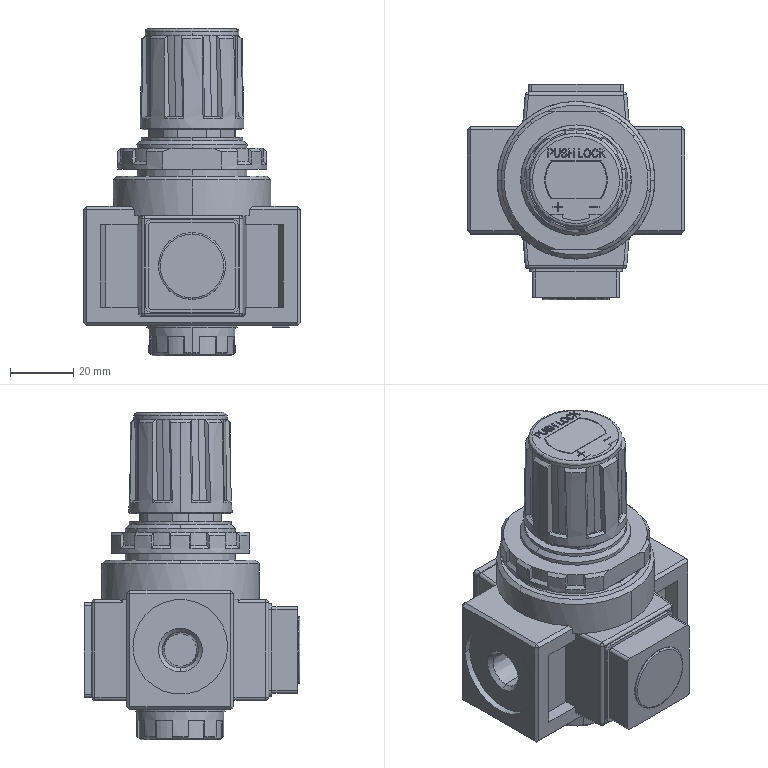Part | SolidWorks | features BaseBody 5 | 5 solids | 618 faces | box 68.8 x 68.4 x 103.9 mm | volume 177481 mm3 | plane 320 | cylinder 131 | spline 100 | cone 67 | commonest cylinder face diameters 2 x34 9 x13 27.5 x9 2.5 x8 26.6 x8 45.5 x8